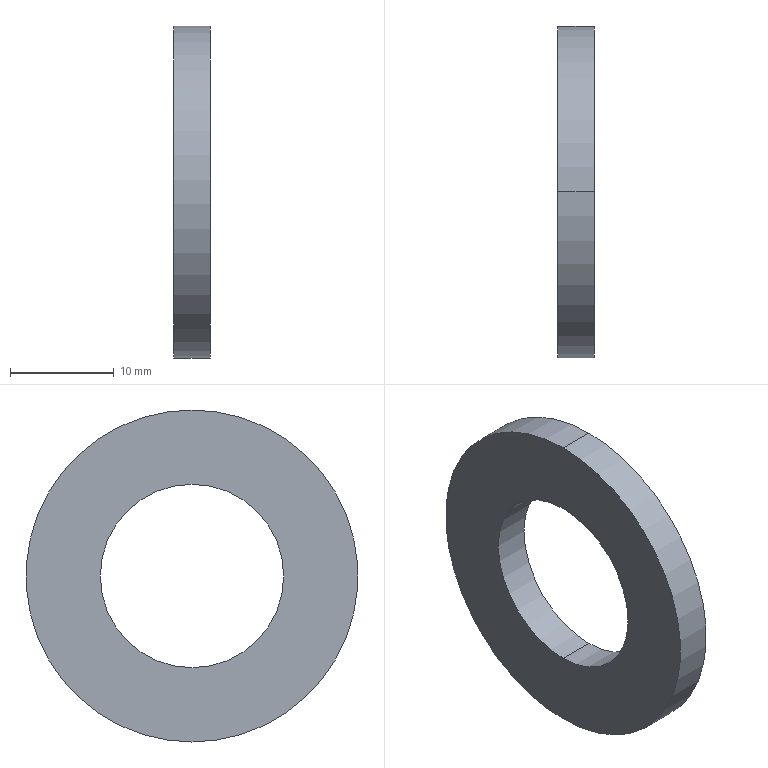Part | STEP file | flat washer narrow_am_B18.22M - Plain washer, 16 mm, narrow | 1 solid | 6 faces | box 3.5 x 32 x 32 mm | volume 1956 mm3 | cylinder 4 | plane 2 | commonest cylinder face diameters 17.68 x2 32 x2
STEP:
#1=CARTESIAN_POINT('',(0.,0.,0.));
#2=DIRECTION('',(0.,0.,1.));
#3=DIRECTION('',(1.,0.,0.));
#4=AXIS2_PLACEMENT_3D('',#1,#2,#3);
#5=CARTESIAN_POINT('',(0.,0.,16.));
#6=VERTEX_POINT('',#5);
#7=CARTESIAN_POINT('',(0.,0.,-16.));
#8=VERTEX_POINT('',#7);
#9=CARTESIAN_POINT('',(0.,0.,0.));
#10=DIRECTION('',(-1.,0.,0.));
#11=DIRECTION('',(0.,0.,1.));
#12=AXIS2_PLACEMENT_3D('',#9,#10,#11);
#13=CIRCLE('',#12,16.);
#14=CARTESIAN_POINT('',(-34.925,0.,0.));
#15=DIRECTION('',(-1.,0.,0.));
#16=DIRECTION('',(0.,0.,1.));
#17=AXIS2_PLACEMENT_3D('',#14,#15,#16);
#18=CYLINDRICAL_SURFACE('',#17,16.);
#19=CARTESIAN_POINT('',(0.,-34.925));
#20=DIRECTION('',(1.,0.));
#21=VECTOR('',#20,1.);
#22=LINE('',#19,#21);
#23=(GEOMETRIC_REPRESENTATION_CONTEXT(2)PARAMETRIC_REPRESENTATION_CONTEXT()REPRESENTATION_CONTEXT('',''));
#24=DEFINITIONAL_REPRESENTATION('',(#22),#23);
#25=PCURVE('',#18,#24);
#26=CARTESIAN_POINT('',(0.,8.84,0.));
#27=DIRECTION('',(-1.,0.,0.));
#28=DIRECTION('',(0.,0.,1.));
#29=AXIS2_PLACEMENT_3D('',#26,#27,#28);
#30=PLANE('',#29);
#31=CARTESIAN_POINT('',(0.,-8.84));
#32=DIRECTION('',(1.,0.));
#33=AXIS2_PLACEMENT_2D('',#31,#32);
#34=CIRCLE('',#33,16.);
#35=(GEOMETRIC_REPRESENTATION_CONTEXT(2)PARAMETRIC_REPRESENTATION_CONTEXT()REPRESENTATION_CONTEXT('',''));
#36=DEFINITIONAL_REPRESENTATION('',(#34),#35);
#37=PCURVE('',#30,#36);
#38=SURFACE_CURVE('',#13,(#25,#37),.PCURVE_S1.);
#39=EDGE_CURVE('',#6,#8,#38,.T.);
#40=ORIENTED_EDGE('',*,*,#39,.T.);
#41=CARTESIAN_POINT('',(-3.5,0.,-16.));
#42=VERTEX_POINT('',#41);
#43=CARTESIAN_POINT('',(-34.925,0.,-16.));
#44=DIRECTION('',(-1.,0.,0.));
#45=VECTOR('',#44,1.);
#46=LINE('',#43,#45);
#47=CARTESIAN_POINT('',(3.142,0.));
#48=DIRECTION('',(0.,1.));
#49=VECTOR('',#48,1.);
#50=LINE('',#47,#49);
#51=(GEOMETRIC_REPRESENTATION_CONTEXT(2)PARAMETRIC_REPRESENTATION_CONTEXT()REPRESENTATION_CONTEXT('',''));
#52=DEFINITIONAL_REPRESENTATION('',(#50),#51);
#53=PCURVE('',#18,#52);
#54=CARTESIAN_POINT('',(-34.925,0.,0.));
#55=DIRECTION('',(-1.,0.,0.));
#56=DIRECTION('',(0.,0.,1.));
#57=AXIS2_PLACEMENT_3D('',#54,#55,#56);
#58=CYLINDRICAL_SURFACE('',#57,16.);
#59=CARTESIAN_POINT('',(3.142,0.));
#60=DIRECTION('',(0.,1.));
#61=VECTOR('',#60,1.);
#62=LINE('',#59,#61);
#63=(GEOMETRIC_REPRESENTATION_CONTEXT(2)PARAMETRIC_REPRESENTATION_CONTEXT()REPRESENTATION_CONTEXT('',''));
#64=DEFINITIONAL_REPRESENTATION('',(#62),#63);
#65=PCURVE('',#58,#64);
#66=SURFACE_CURVE('',#46,(#53,#65),.PCURVE_S1.);
#67=EDGE_CURVE('',#8,#42,#66,.T.);
#68=ORIENTED_EDGE('',*,*,#67,.T.);
#69=CARTESIAN_POINT('',(-3.5,0.,16.));
#70=VERTEX_POINT('',#69);
#71=CARTESIAN_POINT('',(-3.5,0.,0.));
#72=DIRECTION('',(-1.,0.,0.));
#73=DIRECTION('',(0.,0.,1.));
#74=AXIS2_PLACEMENT_3D('',#71,#72,#73);
#75=CIRCLE('',#74,16.);
#76=CARTESIAN_POINT('',(0.,-31.425));
#77=DIRECTION('',(1.,0.));
#78=VECTOR('',#77,1.);
#79=LINE('',#76,#78);
#80=(GEOMETRIC_REPRESENTATION_CONTEXT(2)PARAMETRIC_REPRESENTATION_CONTEXT()REPRESENTATION_CONTEXT('',''));
#81=DEFINITIONAL_REPRESENTATION('',(#79),#80);
#82=PCURVE('',#18,#81);
#83=CARTESIAN_POINT('',(-3.5,16.,0.));
#84=DIRECTION('',(1.,0.,0.));
#85=DIRECTION('',(0.,0.,-1.));
#86=AXIS2_PLACEMENT_3D('',#83,#84,#85);
#87=PLANE('',#86);
#88=CARTESIAN_POINT('',(-16.,-16.));
#89=CARTESIAN_POINT('',(-16.,11.713));
#90=CARTESIAN_POINT('',(8.,-2.144));
#91=CARTESIAN_POINT('',(32.,-16.));
#92=CARTESIAN_POINT('',(8.,-29.856));
#93=CARTESIAN_POINT('',(-16.,-43.713));
#94=CARTESIAN_POINT('',(-16.,-16.));
#95=(BOUNDED_CURVE()B_SPLINE_CURVE(2,(#88,#89,#90,#91,#92,#93,#94),.UNSPECIFIED.,.T.,.F.)B_SPLINE_CURVE_WITH_KNOTS((1,2,2,2,2,1),(-2.094,0.,2.094,4.189,6.283,8.378),.UNSPECIFIED.)CURVE()GEOMETRIC_REPRESENTATION_ITEM()RATIONAL_B_SPLINE_CURVE((1.,0.5,1.,0.5,1.,0.5,1.))REPRESENTATION_ITEM(''));
#96=(GEOMETRIC_REPRESENTATION_CONTEXT(2)PARAMETRIC_REPRESENTATION_CONTEXT()REPRESENTATION_CONTEXT('',''));
#97=DEFINITIONAL_REPRESENTATION('',(#95),#96);
#98=PCURVE('',#87,#97);
#99=SURFACE_CURVE('',#75,(#82,#98),.PCURVE_S1.);
#100=EDGE_CURVE('',#70,#42,#99,.T.);
#101=ORIENTED_EDGE('',*,*,#100,.F.);
#102=CARTESIAN_POINT('',(-34.925,0.,16.));
#103=DIRECTION('',(-1.,0.,0.));
#104=VECTOR('',#103,1.);
#105=LINE('',#102,#104);
#106=CARTESIAN_POINT('',(0.,0.));
#107=DIRECTION('',(0.,1.));
#108=VECTOR('',#107,1.);
#109=LINE('',#106,#108);
#110=(GEOMETRIC_REPRESENTATION_CONTEXT(2)PARAMETRIC_REPRESENTATION_CONTEXT()REPRESENTATION_CONTEXT('',''));
#111=DEFINITIONAL_REPRESENTATION('',(#109),#110);
#112=PCURVE('',#18,#111);
#113=CARTESIAN_POINT('',(6.283,0.));
#114=DIRECTION('',(0.,1.));
#115=VECTOR('',#114,1.);
#116=LINE('',#113,#115);
#117=(GEOMETRIC_REPRESENTATION_CONTEXT(2)PARAMETRIC_REPRESENTATION_CONTEXT()REPRESENTATION_CONTEXT('',''));
#118=DEFINITIONAL_REPRESENTATION('',(#116),#117);
#119=PCURVE('',#58,#118);
#120=SURFACE_CURVE('',#105,(#112,#119),.PCURVE_S1.);
#121=EDGE_CURVE('',#6,#70,#120,.T.);
#122=ORIENTED_EDGE('',*,*,#121,.F.);
#123=EDGE_LOOP('',(#40,#68,#101,#122));
#124=FACE_BOUND('',#123,.T.);
#125=ADVANCED_FACE('',(#124),#18,.T.);
#126=CARTESIAN_POINT('',(0.,0.,8.84));
#127=VERTEX_POINT('',#126);
#128=CARTESIAN_POINT('',(-3.5,0.,8.84));
#129=VERTEX_POINT('',#128);
#130=CARTESIAN_POINT('',(-34.925,0.,8.84));
#131=DIRECTION('',(-1.,0.,0.));
#132=VECTOR('',#131,1.);
#133=LINE('',#130,#132);
#134=CARTESIAN_POINT('',(-34.925,0.,0.));
#135=DIRECTION('',(-1.,0.,0.));
#136=DIRECTION('',(0.,0.,1.));
#137=AXIS2_PLACEMENT_3D('',#134,#135,#136);
#138=CYLINDRICAL_SURFACE('',#137,8.84);
#139=CARTESIAN_POINT('',(6.283,0.));
#140=DIRECTION('',(0.,1.));
#141=VECTOR('',#140,1.);
#142=LINE('',#139,#141);
#143=(GEOMETRIC_REPRESENTATION_CONTEXT(2)PARAMETRIC_REPRESENTATION_CONTEXT()REPRESENTATION_CONTEXT('',''));
#144=DEFINITIONAL_REPRESENTATION('',(#142),#143);
#145=PCURVE('',#138,#144);
#146=CARTESIAN_POINT('',(-34.925,0.,0.));
#147=DIRECTION('',(-1.,0.,0.));
#148=DIRECTION('',(0.,0.,1.));
#149=AXIS2_PLACEMENT_3D('',#146,#147,#148);
#150=CYLINDRICAL_SURFACE('',#149,8.84);
#151=CARTESIAN_POINT('',(0.,0.));
#152=DIRECTION('',(0.,1.));
#153=VECTOR('',#152,1.);
#154=LINE('',#151,#153);
#155=(GEOMETRIC_REPRESENTATION_CONTEXT(2)PARAMETRIC_REPRESENTATION_CONTEXT()REPRESENTATION_CONTEXT('',''));
#156=DEFINITIONAL_REPRESENTATION('',(#154),#155);
#157=PCURVE('',#150,#156);
#158=SURFACE_CURVE('',#133,(#145,#157),.PCURVE_S1.);
#159=EDGE_CURVE('',#127,#129,#158,.T.);
#160=ORIENTED_EDGE('',*,*,#159,.T.);
#161=CARTESIAN_POINT('',(-3.5,0.,-8.84));
#162=VERTEX_POINT('',#161);
#163=CARTESIAN_POINT('',(-3.5,0.,0.));
#164=DIRECTION('',(-1.,0.,0.));
#165=DIRECTION('',(0.,0.,1.));
#166=AXIS2_PLACEMENT_3D('',#163,#164,#165);
#167=CIRCLE('',#166,8.84);
#168=CARTESIAN_POINT('',(0.,-31.425));
#169=DIRECTION('',(1.,0.));
#170=VECTOR('',#169,1.);
#171=LINE('',#168,#170);
#172=(GEOMETRIC_REPRESENTATION_CONTEXT(2)PARAMETRIC_REPRESENTATION_CONTEXT()REPRESENTATION_CONTEXT('',''));
#173=DEFINITIONAL_REPRESENTATION('',(#171),#172);
#174=PCURVE('',#138,#173);
#175=CARTESIAN_POINT('',(-8.84,-16.));
#176=CARTESIAN_POINT('',(-8.84,-0.6887));
#177=CARTESIAN_POINT('',(4.42,-8.344));
#178=CARTESIAN_POINT('',(17.68,-16.));
#179=CARTESIAN_POINT('',(4.42,-23.656));
#180=CARTESIAN_POINT('',(-8.84,-31.311));
#181=CARTESIAN_POINT('',(-8.84,-16.));
#182=(BOUNDED_CURVE()B_SPLINE_CURVE(2,(#175,#176,#177,#178,#179,#180,#181),.UNSPECIFIED.,.T.,.F.)B_SPLINE_CURVE_WITH_KNOTS((1,2,2,2,2,1),(-2.094,0.,2.094,4.189,6.283,8.378),.UNSPECIFIED.)CURVE()GEOMETRIC_REPRESENTATION_ITEM()RATIONAL_B_SPLINE_CURVE((1.,0.5,1.,0.5,1.,0.5,1.))REPRESENTATION_ITEM(''));
#183=(GEOMETRIC_REPRESENTATION_CONTEXT(2)PARAMETRIC_REPRESENTATION_CONTEXT()REPRESENTATION_CONTEXT('',''));
#184=DEFINITIONAL_REPRESENTATION('',(#182),#183);
#185=PCURVE('',#87,#184);
#186=SURFACE_CURVE('',#167,(#174,#185),.PCURVE_S1.);
#187=EDGE_CURVE('',#162,#129,#186,.T.);
#188=ORIENTED_EDGE('',*,*,#187,.F.);
#189=CARTESIAN_POINT('',(0.,0.,-8.84));
#190=VERTEX_POINT('',#189);
#191=CARTESIAN_POINT('',(-34.925,0.,-8.84));
#192=DIRECTION('',(-1.,0.,0.));
#193=VECTOR('',#192,1.);
#194=LINE('',#191,#193);
#195=CARTESIAN_POINT('',(3.142,0.));
#196=DIRECTION('',(0.,1.));
#197=VECTOR('',#196,1.);
#198=LINE('',#195,#197);
#199=(GEOMETRIC_REPRESENTATION_CONTEXT(2)PARAMETRIC_REPRESENTATION_CONTEXT()REPRESENTATION_CONTEXT('',''));
#200=DEFINITIONAL_REPRESENTATION('',(#198),#199);
#201=PCURVE('',#138,#200);
#202=CARTESIAN_POINT('',(3.142,0.));
#203=DIRECTION('',(0.,1.));
#204=VECTOR('',#203,1.);
#205=LINE('',#202,#204);
#206=(GEOMETRIC_REPRESENTATION_CONTEXT(2)PARAMETRIC_REPRESENTATION_CONTEXT()REPRESENTATION_CONTEXT('',''));
#207=DEFINITIONAL_REPRESENTATION('',(#205),#206);
#208=PCURVE('',#150,#207);
#209=SURFACE_CURVE('',#194,(#201,#208),.PCURVE_S1.);
#210=EDGE_CURVE('',#190,#162,#209,.T.);
#211=ORIENTED_EDGE('',*,*,#210,.F.);
#212=CARTESIAN_POINT('',(0.,0.,0.));
#213=DIRECTION('',(-1.,0.,0.));
#214=DIRECTION('',(0.,0.,1.));
#215=AXIS2_PLACEMENT_3D('',#212,#213,#214);
#216=CIRCLE('',#215,8.84);
#217=CARTESIAN_POINT('',(0.,-34.925));
#218=DIRECTION('',(1.,0.));
#219=VECTOR('',#218,1.);
#220=LINE('',#217,#219);
#221=(GEOMETRIC_REPRESENTATION_CONTEXT(2)PARAMETRIC_REPRESENTATION_CONTEXT()REPRESENTATION_CONTEXT('',''));
#222=DEFINITIONAL_REPRESENTATION('',(#220),#221);
#223=PCURVE('',#138,#222);
#224=CARTESIAN_POINT('',(0.,-8.84));
#225=DIRECTION('',(1.,0.));
#226=AXIS2_PLACEMENT_2D('',#224,#225);
#227=CIRCLE('',#226,8.84);
#228=(GEOMETRIC_REPRESENTATION_CONTEXT(2)PARAMETRIC_REPRESENTATION_CONTEXT()REPRESENTATION_CONTEXT('',''));
#229=DEFINITIONAL_REPRESENTATION('',(#227),#228);
#230=PCURVE('',#30,#229);
#231=SURFACE_CURVE('',#216,(#223,#230),.PCURVE_S1.);
#232=EDGE_CURVE('',#190,#127,#231,.T.);
#233=ORIENTED_EDGE('',*,*,#232,.T.);
#234=EDGE_LOOP('',(#160,#188,#211,#233));
#235=FACE_BOUND('',#234,.F.);
#236=ADVANCED_FACE('',(#235),#138,.F.);
#237=CARTESIAN_POINT('',(-3.5,0.,0.));
#238=DIRECTION('',(-1.,0.,0.));
#239=DIRECTION('',(0.,0.,1.));
#240=AXIS2_PLACEMENT_3D('',#237,#238,#239);
#241=CIRCLE('',#240,8.84);
#242=CARTESIAN_POINT('',(0.,-31.425));
#243=DIRECTION('',(1.,0.));
#244=VECTOR('',#243,1.);
#245=LINE('',#242,#244);
#246=(GEOMETRIC_REPRESENTATION_CONTEXT(2)PARAMETRIC_REPRESENTATION_CONTEXT()REPRESENTATION_CONTEXT('',''));
#247=DEFINITIONAL_REPRESENTATION('',(#245),#246);
#248=PCURVE('',#150,#247);
#249=CARTESIAN_POINT('',(-8.84,-16.));
#250=CARTESIAN_POINT('',(-8.84,-0.6887));
#251=CARTESIAN_POINT('',(4.42,-8.344));
#252=CARTESIAN_POINT('',(17.68,-16.));
#253=CARTESIAN_POINT('',(4.42,-23.656));
#254=CARTESIAN_POINT('',(-8.84,-31.311));
#255=CARTESIAN_POINT('',(-8.84,-16.));
#256=(BOUNDED_CURVE()B_SPLINE_CURVE(2,(#249,#250,#251,#252,#253,#254,#255),.UNSPECIFIED.,.T.,.F.)B_SPLINE_CURVE_WITH_KNOTS((1,2,2,2,2,1),(-2.094,0.,2.094,4.189,6.283,8.378),.UNSPECIFIED.)CURVE()GEOMETRIC_REPRESENTATION_ITEM()RATIONAL_B_SPLINE_CURVE((1.,0.5,1.,0.5,1.,0.5,1.))REPRESENTATION_ITEM(''));
#257=(GEOMETRIC_REPRESENTATION_CONTEXT(2)PARAMETRIC_REPRESENTATION_CONTEXT()REPRESENTATION_CONTEXT('',''));
#258=DEFINITIONAL_REPRESENTATION('',(#256),#257);
#259=PCURVE('',#87,#258);
#260=SURFACE_CURVE('',#241,(#248,#259),.PCURVE_S1.);
#261=EDGE_CURVE('',#129,#162,#260,.T.);
#262=ORIENTED_EDGE('',*,*,#261,.F.);
#263=ORIENTED_EDGE('',*,*,#159,.F.);
#264=CARTESIAN_POINT('',(0.,0.,0.));
#265=DIRECTION('',(-1.,0.,0.));
#266=DIRECTION('',(0.,0.,1.));
#267=AXIS2_PLACEMENT_3D('',#264,#265,#266);
#268=CIRCLE('',#267,8.84);
#269=CARTESIAN_POINT('',(0.,-34.925));
#270=DIRECTION('',(1.,0.));
#271=VECTOR('',#270,1.);
#272=LINE('',#269,#271);
#273=(GEOMETRIC_REPRESENTATION_CONTEXT(2)PARAMETRIC_REPRESENTATION_CONTEXT()REPRESENTATION_CONTEXT('',''));
#274=DEFINITIONAL_REPRESENTATION('',(#272),#273);
#275=PCURVE('',#150,#274);
#276=CARTESIAN_POINT('',(0.,-8.84));
#277=DIRECTION('',(1.,0.));
#278=AXIS2_PLACEMENT_2D('',#276,#277);
#279=CIRCLE('',#278,8.84);
#280=(GEOMETRIC_REPRESENTATION_CONTEXT(2)PARAMETRIC_REPRESENTATION_CONTEXT()REPRESENTATION_CONTEXT('',''));
#281=DEFINITIONAL_REPRESENTATION('',(#279),#280);
#282=PCURVE('',#30,#281);
#283=SURFACE_CURVE('',#268,(#275,#282),.PCURVE_S1.);
#284=EDGE_CURVE('',#127,#190,#283,.T.);
#285=ORIENTED_EDGE('',*,*,#284,.T.);
#286=ORIENTED_EDGE('',*,*,#210,.T.);
#287=EDGE_LOOP('',(#262,#263,#285,#286));
#288=FACE_BOUND('',#287,.F.);
#289=ADVANCED_FACE('',(#288),#150,.F.);
#290=ORIENTED_EDGE('',*,*,#39,.F.);
#291=CARTESIAN_POINT('',(0.,0.,0.));
#292=DIRECTION('',(-1.,0.,0.));
#293=DIRECTION('',(0.,0.,1.));
#294=AXIS2_PLACEMENT_3D('',#291,#292,#293);
#295=CIRCLE('',#294,16.);
#296=CARTESIAN_POINT('',(0.,-8.84));
#297=DIRECTION('',(1.,0.));
#298=AXIS2_PLACEMENT_2D('',#296,#297);
#299=CIRCLE('',#298,16.);
#300=(GEOMETRIC_REPRESENTATION_CONTEXT(2)PARAMETRIC_REPRESENTATION_CONTEXT()REPRESENTATION_CONTEXT('',''));
#301=DEFINITIONAL_REPRESENTATION('',(#299),#300);
#302=PCURVE('',#30,#301);
#303=CARTESIAN_POINT('',(0.,-34.925));
#304=DIRECTION('',(1.,0.));
#305=VECTOR('',#304,1.);
#306=LINE('',#303,#305);
#307=(GEOMETRIC_REPRESENTATION_CONTEXT(2)PARAMETRIC_REPRESENTATION_CONTEXT()REPRESENTATION_CONTEXT('',''));
#308=DEFINITIONAL_REPRESENTATION('',(#306),#307);
#309=PCURVE('',#58,#308);
#310=SURFACE_CURVE('',#295,(#302,#309),.PCURVE_S1.);
#311=EDGE_CURVE('',#8,#6,#310,.T.);
#312=ORIENTED_EDGE('',*,*,#311,.F.);
#313=EDGE_LOOP('',(#290,#312));
#314=FACE_BOUND('',#313,.T.);
#315=ORIENTED_EDGE('',*,*,#284,.T.);
#316=ORIENTED_EDGE('',*,*,#232,.T.);
#317=EDGE_LOOP('',(#315,#316));
#318=FACE_BOUND('',#317,.T.);
#319=ADVANCED_FACE('',(#314,#318),#30,.F.);
#320=ORIENTED_EDGE('',*,*,#67,.F.);
#321=ORIENTED_EDGE('',*,*,#311,.T.);
#322=ORIENTED_EDGE('',*,*,#121,.T.);
#323=CARTESIAN_POINT('',(-3.5,0.,0.));
#324=DIRECTION('',(-1.,0.,0.));
#325=DIRECTION('',(0.,0.,1.));
#326=AXIS2_PLACEMENT_3D('',#323,#324,#325);
#327=CIRCLE('',#326,16.);
#328=CARTESIAN_POINT('',(0.,-31.425));
#329=DIRECTION('',(1.,0.));
#330=VECTOR('',#329,1.);
#331=LINE('',#328,#330);
#332=(GEOMETRIC_REPRESENTATION_CONTEXT(2)PARAMETRIC_REPRESENTATION_CONTEXT()REPRESENTATION_CONTEXT('',''));
#333=DEFINITIONAL_REPRESENTATION('',(#331),#332);
#334=PCURVE('',#58,#333);
#335=CARTESIAN_POINT('',(-16.,-16.));
#336=CARTESIAN_POINT('',(-16.,11.713));
#337=CARTESIAN_POINT('',(8.,-2.144));
#338=CARTESIAN_POINT('',(32.,-16.));
#339=CARTESIAN_POINT('',(8.,-29.856));
#340=CARTESIAN_POINT('',(-16.,-43.713));
#341=CARTESIAN_POINT('',(-16.,-16.));
#342=(BOUNDED_CURVE()B_SPLINE_CURVE(2,(#335,#336,#337,#338,#339,#340,#341),.UNSPECIFIED.,.T.,.F.)B_SPLINE_CURVE_WITH_KNOTS((1,2,2,2,2,1),(-2.094,0.,2.094,4.189,6.283,8.378),.UNSPECIFIED.)CURVE()GEOMETRIC_REPRESENTATION_ITEM()RATIONAL_B_SPLINE_CURVE((1.,0.5,1.,0.5,1.,0.5,1.))REPRESENTATION_ITEM(''));
#343=(GEOMETRIC_REPRESENTATION_CONTEXT(2)PARAMETRIC_REPRESENTATION_CONTEXT()REPRESENTATION_CONTEXT('',''));
#344=DEFINITIONAL_REPRESENTATION('',(#342),#343);
#345=PCURVE('',#87,#344);
#346=SURFACE_CURVE('',#327,(#334,#345),.PCURVE_S1.);
#347=EDGE_CURVE('',#42,#70,#346,.T.);
#348=ORIENTED_EDGE('',*,*,#347,.F.);
#349=EDGE_LOOP('',(#320,#321,#322,#348));
#350=FACE_BOUND('',#349,.T.);
#351=ADVANCED_FACE('',(#350),#58,.T.);
#352=ORIENTED_EDGE('',*,*,#261,.F.);
#353=ORIENTED_EDGE('',*,*,#187,.F.);
#354=EDGE_LOOP('',(#352,#353));
#355=FACE_BOUND('',#354,.T.);
#356=ORIENTED_EDGE('',*,*,#100,.T.);
#357=ORIENTED_EDGE('',*,*,#347,.T.);
#358=EDGE_LOOP('',(#356,#357));
#359=FACE_BOUND('',#358,.T.);
#360=ADVANCED_FACE('',(#355,#359),#87,.F.);
#361=CLOSED_SHELL('',(#125,#236,#289,#319,#351,#360));
#362=MANIFOLD_SOLID_BREP('',#361);
#363=(LENGTH_UNIT()NAMED_UNIT(*)SI_UNIT(.MILLI.,.METRE.));
#364=UNCERTAINTY_MEASURE_WITH_UNIT(LENGTH_MEASURE(0.0000001),#363,'','');
#365=(NAMED_UNIT(*)PLANE_ANGLE_UNIT()SI_UNIT($,.RADIAN.));
#366=(NAMED_UNIT(*)SI_UNIT($,.STERADIAN.)SOLID_ANGLE_UNIT());
#367=(GEOMETRIC_REPRESENTATION_CONTEXT(3)GLOBAL_UNCERTAINTY_ASSIGNED_CONTEXT((#364))GLOBAL_UNIT_ASSIGNED_CONTEXT((#363,#365,#366))REPRESENTATION_CONTEXT('',''));
#368=ADVANCED_BREP_SHAPE_REPRESENTATION('',(#4,#362),#367);